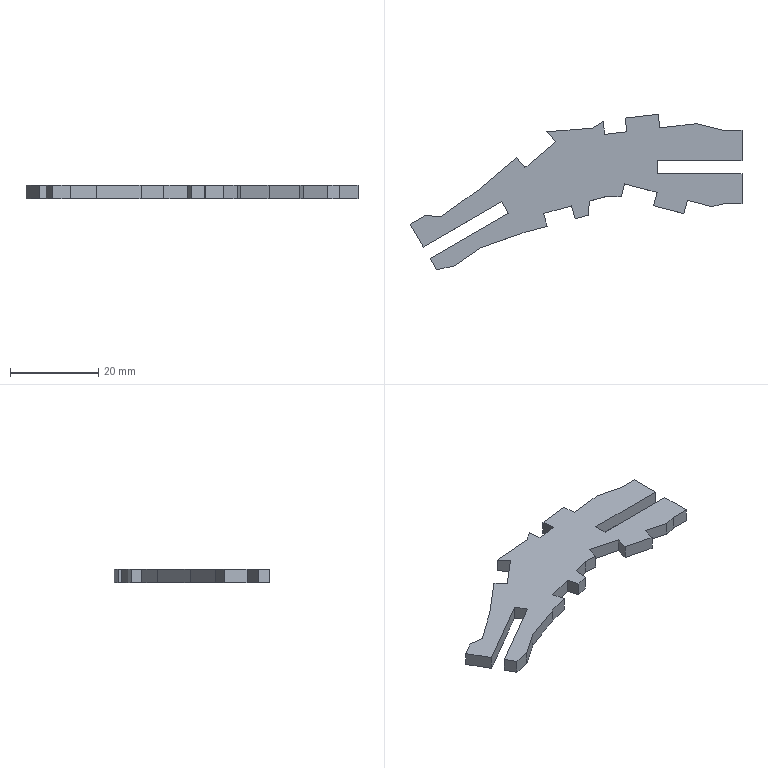Part | SolidWorks | features BaseBody 1 | 1 solid | 48 faces | box 75.297 x 35.268 x 3 mm | volume 3149 mm3 | plane 48
STEP:
#1=CARTESIAN_POINT('',(-41.672,11.926,-1.5));
#2=VERTEX_POINT('',#1);
#3=CARTESIAN_POINT('',(-45.861,11.926,-1.5));
#4=VERTEX_POINT('',#3);
#5=CARTESIAN_POINT('',(0.,11.926,-1.5));
#6=DIRECTION('',(-1.,0.,0.));
#7=VECTOR('',#6,1000.);
#8=LINE('',#5,#7);
#9=EDGE_CURVE('',#2,#4,#8,.T.);
#10=ORIENTED_EDGE('',*,*,#9,.F.);
#11=CARTESIAN_POINT('',(-41.672,5.086,-1.5));
#12=VERTEX_POINT('',#11);
#13=CARTESIAN_POINT('',(-41.672,0.,-1.5));
#14=DIRECTION('',(0.,1.,0.));
#15=VECTOR('',#14,1000.);
#16=LINE('',#13,#15);
#17=EDGE_CURVE('',#12,#2,#16,.T.);
#18=ORIENTED_EDGE('',*,*,#17,.F.);
#19=CARTESIAN_POINT('',(-60.886,5.086,-1.5));
#20=VERTEX_POINT('',#19);
#21=CARTESIAN_POINT('',(0.,5.086,-1.5));
#22=DIRECTION('',(1.,0.,0.));
#23=VECTOR('',#22,1000.);
#24=LINE('',#21,#23);
#25=EDGE_CURVE('',#20,#12,#24,.T.);
#26=ORIENTED_EDGE('',*,*,#25,.F.);
#27=CARTESIAN_POINT('',(-60.886,2.088,-1.5));
#28=VERTEX_POINT('',#27);
#29=CARTESIAN_POINT('',(-60.886,0.,-1.5));
#30=DIRECTION('',(0.,1.,0.));
#31=VECTOR('',#30,1000.);
#32=LINE('',#29,#31);
#33=EDGE_CURVE('',#28,#20,#32,.T.);
#34=ORIENTED_EDGE('',*,*,#33,.F.);
#35=CARTESIAN_POINT('',(-41.672,2.088,-1.5));
#36=VERTEX_POINT('',#35);
#37=CARTESIAN_POINT('',(0.,2.088,-1.5));
#38=DIRECTION('',(-1.,0.,0.));
#39=VECTOR('',#38,1000.);
#40=LINE('',#37,#39);
#41=EDGE_CURVE('',#36,#28,#40,.T.);
#42=ORIENTED_EDGE('',*,*,#41,.F.);
#43=CARTESIAN_POINT('',(-41.672,-4.747,-1.5));
#44=VERTEX_POINT('',#43);
#45=CARTESIAN_POINT('',(-41.672,0.,-1.5));
#46=DIRECTION('',(0.,1.,0.));
#47=VECTOR('',#46,1000.);
#48=LINE('',#45,#47);
#49=EDGE_CURVE('',#44,#36,#48,.T.);
#50=ORIENTED_EDGE('',*,*,#49,.F.);
#51=CARTESIAN_POINT('',(-45.859,-4.748,-1.5));
#52=VERTEX_POINT('',#51);
#53=CARTESIAN_POINT('',(0.0009716,-4.738,-1.5));
#54=DIRECTION('',(1.,0.000205,0.));
#55=VECTOR('',#54,1000.);
#56=LINE('',#53,#55);
#57=EDGE_CURVE('',#52,#44,#56,.T.);
#58=ORIENTED_EDGE('',*,*,#57,.F.);
#59=CARTESIAN_POINT('',(-48.55,-5.367,-1.5));
#60=VERTEX_POINT('',#59);
#61=CARTESIAN_POINT('',(-1.268,5.512,-1.5));
#62=DIRECTION('',(0.9745,0.2242,0.));
#63=VECTOR('',#62,1000.);
#64=LINE('',#61,#63);
#65=EDGE_CURVE('',#60,#52,#64,.T.);
#66=ORIENTED_EDGE('',*,*,#65,.F.);
#67=CARTESIAN_POINT('',(-54.059,-3.94,-1.5));
#68=VERTEX_POINT('',#67);
#69=CARTESIAN_POINT('',(-4.355,-16.813,-1.5));
#70=DIRECTION('',(0.9681,-0.2507,0.));
#71=VECTOR('',#70,1000.);
#72=LINE('',#69,#71);
#73=EDGE_CURVE('',#68,#60,#72,.T.);
#74=ORIENTED_EDGE('',*,*,#73,.F.);
#75=CARTESIAN_POINT('',(-54.841,-6.951,-1.5));
#76=VERTEX_POINT('',#75);
#77=CARTESIAN_POINT('',(-49.682,12.907,-1.5));
#78=DIRECTION('',(0.2514,0.9679,0.));
#79=VECTOR('',#78,1000.);
#80=LINE('',#77,#79);
#81=EDGE_CURVE('',#76,#68,#80,.T.);
#82=ORIENTED_EDGE('',*,*,#81,.F.);
#83=CARTESIAN_POINT('',(-61.711,-5.166,-1.5));
#84=VERTEX_POINT('',#83);
#85=CARTESIAN_POINT('',(-5.159,-19.858,-1.5));
#86=DIRECTION('',(0.9679,-0.2514,0.));
#87=VECTOR('',#86,1000.);
#88=LINE('',#85,#87);
#89=EDGE_CURVE('',#84,#76,#88,.T.);
#90=ORIENTED_EDGE('',*,*,#89,.F.);
#91=CARTESIAN_POINT('',(-60.926,-2.144,-1.5));
#92=VERTEX_POINT('',#91);
#93=CARTESIAN_POINT('',(-56.552,14.692,-1.5));
#94=DIRECTION('',(-0.2514,-0.9679,0.));
#95=VECTOR('',#94,1000.);
#96=LINE('',#93,#95);
#97=EDGE_CURVE('',#92,#84,#96,.T.);
#98=ORIENTED_EDGE('',*,*,#97,.F.);
#99=CARTESIAN_POINT('',(-68.318,-0.224,-1.5));
#100=VERTEX_POINT('',#99);
#101=CARTESIAN_POINT('',(-4.372,-16.833,-1.5));
#102=DIRECTION('',(0.9679,-0.2514,0.));
#103=VECTOR('',#102,1000.);
#104=LINE('',#101,#103);
#105=EDGE_CURVE('',#100,#92,#104,.T.);
#106=ORIENTED_EDGE('',*,*,#105,.F.);
#107=CARTESIAN_POINT('',(-69.072,-3.126,-1.5));
#108=VERTEX_POINT('',#107);
#109=CARTESIAN_POINT('',(-63.946,16.609,-1.5));
#110=DIRECTION('',(0.2514,0.9679,0.));
#111=VECTOR('',#110,1000.);
#112=LINE('',#109,#111);
#113=EDGE_CURVE('',#108,#100,#112,.T.);
#114=ORIENTED_EDGE('',*,*,#113,.F.);
#115=CARTESIAN_POINT('',(-72.167,-3.005,-1.5));
#116=VERTEX_POINT('',#115);
#117=CARTESIAN_POINT('',(-0.2275,-5.818,-1.5));
#118=DIRECTION('',(0.9992,-0.03907,0.));
#119=VECTOR('',#118,1000.);
#120=LINE('',#117,#119);
#121=EDGE_CURVE('',#116,#108,#120,.T.);
#122=ORIENTED_EDGE('',*,*,#121,.F.);
#123=CARTESIAN_POINT('',(-76.273,-4.118,-1.5));
#124=VERTEX_POINT('',#123);
#125=CARTESIAN_POINT('',(-4.178,15.419,-1.5));
#126=DIRECTION('',(0.9652,0.2616,0.));
#127=VECTOR('',#126,1000.);
#128=LINE('',#125,#127);
#129=EDGE_CURVE('',#124,#116,#128,.T.);
#130=ORIENTED_EDGE('',*,*,#129,.F.);
#131=CARTESIAN_POINT('',(-76.559,-7.3,-1.5));
#132=VERTEX_POINT('',#131);
#133=CARTESIAN_POINT('',(-75.296,6.762,-1.5));
#134=DIRECTION('',(0.08944,0.996,0.));
#135=VECTOR('',#134,1000.);
#136=LINE('',#133,#135);
#137=EDGE_CURVE('',#132,#124,#136,.T.);
#138=ORIENTED_EDGE('',*,*,#137,.F.);
#139=CARTESIAN_POINT('',(-79.538,-8.108,-1.5));
#140=VERTEX_POINT('',#139);
#141=CARTESIAN_POINT('',(-3.4,12.538,-1.5));
#142=DIRECTION('',(0.9651,0.2617,0.));
#143=VECTOR('',#142,1000.);
#144=LINE('',#141,#143);
#145=EDGE_CURVE('',#140,#132,#144,.T.);
#146=ORIENTED_EDGE('',*,*,#145,.F.);
#147=CARTESIAN_POINT('',(-80.322,-5.216,-1.5));
#148=VERTEX_POINT('',#147);
#149=CARTESIAN_POINT('',(-76.137,-20.649,-1.5));
#150=DIRECTION('',(0.2617,-0.9651,0.));
#151=VECTOR('',#150,1000.);
#152=LINE('',#149,#151);
#153=EDGE_CURVE('',#148,#140,#152,.T.);
#154=ORIENTED_EDGE('',*,*,#153,.F.);
#155=CARTESIAN_POINT('',(-86.653,-6.933,-1.5));
#156=VERTEX_POINT('',#155);
#157=CARTESIAN_POINT('',(-4.185,15.433,-1.5));
#158=DIRECTION('',(0.9651,0.2617,0.));
#159=VECTOR('',#158,1000.);
#160=LINE('',#157,#159);
#161=EDGE_CURVE('',#156,#148,#160,.T.);
#162=ORIENTED_EDGE('',*,*,#161,.F.);
#163=CARTESIAN_POINT('',(-85.869,-9.824,-1.5));
#164=VERTEX_POINT('',#163);
#165=CARTESIAN_POINT('',(-82.468,-22.366,-1.5));
#166=DIRECTION('',(-0.2617,0.9651,0.));
#167=VECTOR('',#166,1000.);
#168=LINE('',#165,#167);
#169=EDGE_CURVE('',#164,#156,#168,.T.);
#170=ORIENTED_EDGE('',*,*,#169,.F.);
#171=CARTESIAN_POINT('',(-90.886,-11.184,-1.5));
#172=VERTEX_POINT('',#171);
#173=CARTESIAN_POINT('',(-3.398,12.534,-1.5));
#174=DIRECTION('',(0.9652,0.2617,0.));
#175=VECTOR('',#174,1000.);
#176=LINE('',#173,#175);
#177=EDGE_CURVE('',#172,#164,#176,.T.);
#178=ORIENTED_EDGE('',*,*,#177,.F.);
#179=CARTESIAN_POINT('',(-100.892,-14.726,-1.5));
#180=VERTEX_POINT('',#179);
#181=CARTESIAN_POINT('',(-6.601,18.649,-1.5));
#182=DIRECTION('',(0.9427,0.3337,0.));
#183=VECTOR('',#182,1000.);
#184=LINE('',#181,#183);
#185=EDGE_CURVE('',#180,#172,#184,.T.);
#186=ORIENTED_EDGE('',*,*,#185,.F.);
#187=CARTESIAN_POINT('',(-106.899,-18.818,-1.5));
#188=VERTEX_POINT('',#187);
#189=CARTESIAN_POINT('',(-25.128,36.886,-1.5));
#190=DIRECTION('',(0.8265,0.563,0.));
#191=VECTOR('',#190,1000.);
#192=LINE('',#189,#191);
#193=EDGE_CURVE('',#188,#180,#192,.T.);
#194=ORIENTED_EDGE('',*,*,#193,.F.);
#195=CARTESIAN_POINT('',(-110.937,-19.69,-1.5));
#196=VERTEX_POINT('',#195);
#197=CARTESIAN_POINT('',(-0.8769,4.063,-1.5));
#198=DIRECTION('',(0.9775,0.211,0.));
#199=VECTOR('',#198,1000.);
#200=LINE('',#197,#199);
#201=EDGE_CURVE('',#196,#188,#200,.T.);
#202=ORIENTED_EDGE('',*,*,#201,.F.);
#203=CARTESIAN_POINT('',(-112.426,-17.126,-1.5));
#204=VERTEX_POINT('',#203);
#205=CARTESIAN_POINT('',(-91.52,-53.134,-1.5));
#206=DIRECTION('',(0.5021,-0.8648,0.));
#207=VECTOR('',#206,1000.);
#208=LINE('',#205,#207);
#209=EDGE_CURVE('',#204,#196,#208,.T.);
#210=ORIENTED_EDGE('',*,*,#209,.F.);
#211=CARTESIAN_POINT('',(-94.713,-6.827,-1.5));
#212=VERTEX_POINT('',#211);
#213=CARTESIAN_POINT('',(-20.961,36.052,-1.5));
#214=DIRECTION('',(-0.8645,-0.5026,0.));
#215=VECTOR('',#214,1000.);
#216=LINE('',#213,#215);
#217=EDGE_CURVE('',#212,#204,#216,.T.);
#218=ORIENTED_EDGE('',*,*,#217,.F.);
#219=CARTESIAN_POINT('',(-96.219,-4.237,-1.5));
#220=VERTEX_POINT('',#219);
#221=CARTESIAN_POINT('',(-73.752,-42.88,-1.5));
#222=DIRECTION('',(0.5026,-0.8645,0.));
#223=VECTOR('',#222,1000.);
#224=LINE('',#221,#223);
#225=EDGE_CURVE('',#220,#212,#224,.T.);
#226=ORIENTED_EDGE('',*,*,#225,.F.);
#227=CARTESIAN_POINT('',(-113.938,-14.539,-1.5));
#228=VERTEX_POINT('',#227);
#229=CARTESIAN_POINT('',(-22.467,38.642,-1.5));
#230=DIRECTION('',(0.8645,0.5026,0.));
#231=VECTOR('',#230,1000.);
#232=LINE('',#229,#231);
#233=EDGE_CURVE('',#228,#220,#232,.T.);
#234=ORIENTED_EDGE('',*,*,#233,.F.);
#235=CARTESIAN_POINT('',(-116.969,-9.333,-1.5));
#236=VERTEX_POINT('',#235);
#237=CARTESIAN_POINT('',(-91.405,-53.231,-1.5));
#238=DIRECTION('',(0.5032,-0.8641,0.));
#239=VECTOR('',#238,1000.);
#240=LINE('',#237,#239);
#241=EDGE_CURVE('',#236,#228,#240,.T.);
#242=ORIENTED_EDGE('',*,*,#241,.F.);
#243=CARTESIAN_POINT('',(-113.563,-7.354,-1.5));
#244=VERTEX_POINT('',#243);
#245=CARTESIAN_POINT('',(-25.463,43.829,-1.5));
#246=DIRECTION('',(-0.8647,-0.5023,0.));
#247=VECTOR('',#246,1000.);
#248=LINE('',#245,#247);
#249=EDGE_CURVE('',#244,#236,#248,.T.);
#250=ORIENTED_EDGE('',*,*,#249,.F.);
#251=CARTESIAN_POINT('',(-110.024,-7.716,-1.5));
#252=VERTEX_POINT('',#251);
#253=CARTESIAN_POINT('',(-1.92,-18.772,-1.5));
#254=DIRECTION('',(-0.9948,0.1017,0.));
#255=VECTOR('',#254,1000.);
#256=LINE('',#253,#255);
#257=EDGE_CURVE('',#252,#244,#256,.T.);
#258=ORIENTED_EDGE('',*,*,#257,.F.);
#259=CARTESIAN_POINT('',(-101.517,-1.618,-1.5));
#260=VERTEX_POINT('',#259);
#261=CARTESIAN_POINT('',(-33.689,47.,-1.5));
#262=DIRECTION('',(-0.8128,-0.5826,0.));
#263=VECTOR('',#262,1000.);
#264=LINE('',#261,#263);
#265=EDGE_CURVE('',#260,#252,#264,.T.);
#266=ORIENTED_EDGE('',*,*,#265,.F.);
#267=CARTESIAN_POINT('',(-92.851,5.744,-1.5));
#268=VERTEX_POINT('',#267);
#269=CARTESIAN_POINT('',(-41.755,49.151,-1.5));
#270=DIRECTION('',(-0.7621,-0.6474,0.));
#271=VECTOR('',#270,1000.);
#272=LINE('',#269,#271);
#273=EDGE_CURVE('',#268,#260,#272,.T.);
#274=ORIENTED_EDGE('',*,*,#273,.F.);
#275=CARTESIAN_POINT('',(-90.898,3.44,-1.5));
#276=VERTEX_POINT('',#275);
#277=CARTESIAN_POINT('',(-51.19,-43.398,-1.5));
#278=DIRECTION('',(-0.6467,0.7628,0.));
#279=VECTOR('',#278,1000.);
#280=LINE('',#277,#279);
#281=EDGE_CURVE('',#276,#268,#280,.T.);
#282=ORIENTED_EDGE('',*,*,#281,.F.);
#283=CARTESIAN_POINT('',(-83.964,9.318,-1.5));
#284=VERTEX_POINT('',#283);
#285=CARTESIAN_POINT('',(-39.708,46.838,-1.5));
#286=DIRECTION('',(-0.7628,-0.6467,0.));
#287=VECTOR('',#286,1000.);
#288=LINE('',#285,#287);
#289=EDGE_CURVE('',#284,#276,#288,.T.);
#290=ORIENTED_EDGE('',*,*,#289,.F.);
#291=CARTESIAN_POINT('',(-85.9,11.602,-1.5));
#292=VERTEX_POINT('',#291);
#293=CARTESIAN_POINT('',(-44.256,-37.519,-1.5));
#294=DIRECTION('',(0.6467,-0.7628,0.));
#295=VECTOR('',#294,1000.);
#296=LINE('',#293,#295);
#297=EDGE_CURVE('',#292,#284,#296,.T.);
#298=ORIENTED_EDGE('',*,*,#297,.F.);
#299=CARTESIAN_POINT('',(-75.689,12.418,-1.5));
#300=VERTEX_POINT('',#299);
#301=CARTESIAN_POINT('',(-1.467,18.351,-1.5));
#302=DIRECTION('',(-0.9968,-0.07967,0.));
#303=VECTOR('',#302,1000.);
#304=LINE('',#301,#303);
#305=EDGE_CURVE('',#300,#292,#304,.T.);
#306=ORIENTED_EDGE('',*,*,#305,.F.);
#307=CARTESIAN_POINT('',(-73.15,13.963,-1.5));
#308=VERTEX_POINT('',#307);
#309=CARTESIAN_POINT('',(-25.962,42.673,-1.5));
#310=DIRECTION('',(-0.8543,-0.5198,0.));
#311=VECTOR('',#310,1000.);
#312=LINE('',#309,#311);
#313=EDGE_CURVE('',#308,#300,#312,.T.);
#314=ORIENTED_EDGE('',*,*,#313,.F.);
#315=CARTESIAN_POINT('',(-72.806,11.016,-1.5));
#316=VERTEX_POINT('',#315);
#317=CARTESIAN_POINT('',(-70.559,-8.237,-1.5));
#318=DIRECTION('',(-0.116,0.9933,0.));
#319=VECTOR('',#318,1000.);
#320=LINE('',#317,#319);
#321=EDGE_CURVE('',#316,#308,#320,.T.);
#322=ORIENTED_EDGE('',*,*,#321,.F.);
#323=CARTESIAN_POINT('',(-67.808,11.6,-1.5));
#324=VERTEX_POINT('',#323);
#325=CARTESIAN_POINT('',(-2.248,19.253,-1.5));
#326=DIRECTION('',(-0.9933,-0.116,0.));
#327=VECTOR('',#326,1000.);
#328=LINE('',#325,#327);
#329=EDGE_CURVE('',#324,#316,#328,.T.);
#330=ORIENTED_EDGE('',*,*,#329,.F.);
#331=CARTESIAN_POINT('',(-68.17,14.703,-1.5));
#332=VERTEX_POINT('',#331);
#333=CARTESIAN_POINT('',(-65.555,-7.665,-1.5));
#334=DIRECTION('',(0.1161,-0.9932,0.));
#335=VECTOR('',#334,1000.);
#336=LINE('',#333,#335);
#337=EDGE_CURVE('',#332,#324,#336,.T.);
#338=ORIENTED_EDGE('',*,*,#337,.F.);
#339=CARTESIAN_POINT('',(-60.678,15.579,-1.5));
#340=VERTEX_POINT('',#339);
#341=CARTESIAN_POINT('',(-2.615,22.368,-1.5));
#342=DIRECTION('',(-0.9932,-0.1161,0.));
#343=VECTOR('',#342,1000.);
#344=LINE('',#341,#343);
#345=EDGE_CURVE('',#340,#332,#344,.T.);
#346=ORIENTED_EDGE('',*,*,#345,.F.);
#347=CARTESIAN_POINT('',(-60.315,12.476,-1.5));
#348=VERTEX_POINT('',#347);
#349=CARTESIAN_POINT('',(-58.063,-6.789,-1.5));
#350=DIRECTION('',(-0.1161,0.9932,0.));
#351=VECTOR('',#350,1000.);
#352=LINE('',#349,#351);
#353=EDGE_CURVE('',#348,#340,#352,.T.);
#354=ORIENTED_EDGE('',*,*,#353,.F.);
#355=CARTESIAN_POINT('',(-52.074,13.44,-1.5));
#356=VERTEX_POINT('',#355);
#357=CARTESIAN_POINT('',(-2.253,19.265,-1.5));
#358=DIRECTION('',(-0.9932,-0.1161,0.));
#359=VECTOR('',#358,1000.);
#360=LINE('',#357,#359);
#361=EDGE_CURVE('',#356,#348,#360,.T.);
#362=ORIENTED_EDGE('',*,*,#361,.F.);
#363=CARTESIAN_POINT('',(0.1731,0.7104,-1.5));
#364=DIRECTION('',(-0.9716,0.2367,0.));
#365=VECTOR('',#364,1000.);
#366=LINE('',#363,#365);
#367=EDGE_CURVE('',#4,#356,#366,.T.);
#368=ORIENTED_EDGE('',*,*,#367,.F.);
#369=EDGE_LOOP('',(#10,#18,#26,#34,#42,#50,#58,#66,#74,#82,#90,#98,#106,#114,#122,#130,#138,#146,#154,#162,#170,#178,#186,#194,#202,#210,#218,#226,#234,#242,#250,#258,#266,#274,#282,#290,#298,#306,#314,#322,#330,#338,#346,#354,#362,#368));
#370=FACE_OUTER_BOUND('',#369,.T.);
#371=CARTESIAN_POINT('',(0.,0.,-1.5));
#372=DIRECTION('',(0.,0.,1.));
#373=DIRECTION('',(1.,0.,0.));
#374=AXIS2_PLACEMENT_3D('',#371,#372,#373);
#375=PLANE('',#374);
#376=ADVANCED_FACE('',(#370),#375,.F.);
#377=CARTESIAN_POINT('',(-41.672,11.926,1.5));
#378=VERTEX_POINT('',#377);
#379=CARTESIAN_POINT('',(-45.861,11.926,1.5));
#380=VERTEX_POINT('',#379);
#381=CARTESIAN_POINT('',(0.,11.926,1.5));
#382=DIRECTION('',(-1.,0.,0.));
#383=VECTOR('',#382,1000.);
#384=LINE('',#381,#383);
#385=EDGE_CURVE('',#378,#380,#384,.T.);
#386=ORIENTED_EDGE('',*,*,#385,.T.);
#387=CARTESIAN_POINT('',(-52.074,13.44,1.5));
#388=VERTEX_POINT('',#387);
#389=CARTESIAN_POINT('',(0.1731,0.7104,1.5));
#390=DIRECTION('',(-0.9716,0.2367,0.));
#391=VECTOR('',#390,1000.);
#392=LINE('',#389,#391);
#393=EDGE_CURVE('',#380,#388,#392,.T.);
#394=ORIENTED_EDGE('',*,*,#393,.T.);
#395=CARTESIAN_POINT('',(-60.315,12.476,1.5));
#396=VERTEX_POINT('',#395);
#397=CARTESIAN_POINT('',(-2.253,19.265,1.5));
#398=DIRECTION('',(-0.9932,-0.1161,0.));
#399=VECTOR('',#398,1000.);
#400=LINE('',#397,#399);
#401=EDGE_CURVE('',#388,#396,#400,.T.);
#402=ORIENTED_EDGE('',*,*,#401,.T.);
#403=CARTESIAN_POINT('',(-60.678,15.579,1.5));
#404=VERTEX_POINT('',#403);
#405=CARTESIAN_POINT('',(-58.063,-6.789,1.5));
#406=DIRECTION('',(-0.1161,0.9932,0.));
#407=VECTOR('',#406,1000.);
#408=LINE('',#405,#407);
#409=EDGE_CURVE('',#396,#404,#408,.T.);
#410=ORIENTED_EDGE('',*,*,#409,.T.);
#411=CARTESIAN_POINT('',(-68.17,14.703,1.5));
#412=VERTEX_POINT('',#411);
#413=CARTESIAN_POINT('',(-2.615,22.368,1.5));
#414=DIRECTION('',(-0.9932,-0.1161,0.));
#415=VECTOR('',#414,1000.);
#416=LINE('',#413,#415);
#417=EDGE_CURVE('',#404,#412,#416,.T.);
#418=ORIENTED_EDGE('',*,*,#417,.T.);
#419=CARTESIAN_POINT('',(-67.808,11.6,1.5));
#420=VERTEX_POINT('',#419);
#421=CARTESIAN_POINT('',(-65.555,-7.665,1.5));
#422=DIRECTION('',(0.1161,-0.9932,0.));
#423=VECTOR('',#422,1000.);
#424=LINE('',#421,#423);
#425=EDGE_CURVE('',#412,#420,#424,.T.);
#426=ORIENTED_EDGE('',*,*,#425,.T.);
#427=CARTESIAN_POINT('',(-72.806,11.016,1.5));
#428=VERTEX_POINT('',#427);
#429=CARTESIAN_POINT('',(-2.248,19.253,1.5));
#430=DIRECTION('',(-0.9933,-0.116,0.));
#431=VECTOR('',#430,1000.);
#432=LINE('',#429,#431);
#433=EDGE_CURVE('',#420,#428,#432,.T.);
#434=ORIENTED_EDGE('',*,*,#433,.T.);
#435=CARTESIAN_POINT('',(-73.15,13.963,1.5));
#436=VERTEX_POINT('',#435);
#437=CARTESIAN_POINT('',(-70.559,-8.237,1.5));
#438=DIRECTION('',(-0.116,0.9933,0.));
#439=VECTOR('',#438,1000.);
#440=LINE('',#437,#439);
#441=EDGE_CURVE('',#428,#436,#440,.T.);
#442=ORIENTED_EDGE('',*,*,#441,.T.);
#443=CARTESIAN_POINT('',(-75.689,12.418,1.5));
#444=VERTEX_POINT('',#443);
#445=CARTESIAN_POINT('',(-25.962,42.673,1.5));
#446=DIRECTION('',(-0.8543,-0.5198,0.));
#447=VECTOR('',#446,1000.);
#448=LINE('',#445,#447);
#449=EDGE_CURVE('',#436,#444,#448,.T.);
#450=ORIENTED_EDGE('',*,*,#449,.T.);
#451=CARTESIAN_POINT('',(-85.9,11.602,1.5));
#452=VERTEX_POINT('',#451);
#453=CARTESIAN_POINT('',(-1.467,18.351,1.5));
#454=DIRECTION('',(-0.9968,-0.07967,0.));
#455=VECTOR('',#454,1000.);
#456=LINE('',#453,#455);
#457=EDGE_CURVE('',#444,#452,#456,.T.);
#458=ORIENTED_EDGE('',*,*,#457,.T.);
#459=CARTESIAN_POINT('',(-83.964,9.318,1.5));
#460=VERTEX_POINT('',#459);
#461=CARTESIAN_POINT('',(-44.256,-37.519,1.5));
#462=DIRECTION('',(0.6467,-0.7628,0.));
#463=VECTOR('',#462,1000.);
#464=LINE('',#461,#463);
#465=EDGE_CURVE('',#452,#460,#464,.T.);
#466=ORIENTED_EDGE('',*,*,#465,.T.);
#467=CARTESIAN_POINT('',(-90.898,3.44,1.5));
#468=VERTEX_POINT('',#467);
#469=CARTESIAN_POINT('',(-39.708,46.838,1.5));
#470=DIRECTION('',(-0.7628,-0.6467,0.));
#471=VECTOR('',#470,1000.);
#472=LINE('',#469,#471);
#473=EDGE_CURVE('',#460,#468,#472,.T.);
#474=ORIENTED_EDGE('',*,*,#473,.T.);
#475=CARTESIAN_POINT('',(-92.851,5.744,1.5));
#476=VERTEX_POINT('',#475);
#477=CARTESIAN_POINT('',(-51.19,-43.398,1.5));
#478=DIRECTION('',(-0.6467,0.7628,0.));
#479=VECTOR('',#478,1000.);
#480=LINE('',#477,#479);
#481=EDGE_CURVE('',#468,#476,#480,.T.);
#482=ORIENTED_EDGE('',*,*,#481,.T.);
#483=CARTESIAN_POINT('',(-101.517,-1.618,1.5));
#484=VERTEX_POINT('',#483);
#485=CARTESIAN_POINT('',(-41.755,49.151,1.5));
#486=DIRECTION('',(-0.7621,-0.6474,0.));
#487=VECTOR('',#486,1000.);
#488=LINE('',#485,#487);
#489=EDGE_CURVE('',#476,#484,#488,.T.);
#490=ORIENTED_EDGE('',*,*,#489,.T.);
#491=CARTESIAN_POINT('',(-110.024,-7.716,1.5));
#492=VERTEX_POINT('',#491);
#493=CARTESIAN_POINT('',(-33.689,47.,1.5));
#494=DIRECTION('',(-0.8128,-0.5826,0.));
#495=VECTOR('',#494,1000.);
#496=LINE('',#493,#495);
#497=EDGE_CURVE('',#484,#492,#496,.T.);
#498=ORIENTED_EDGE('',*,*,#497,.T.);
#499=CARTESIAN_POINT('',(-113.563,-7.354,1.5));
#500=VERTEX_POINT('',#499);
#501=CARTESIAN_POINT('',(-1.92,-18.772,1.5));
#502=DIRECTION('',(-0.9948,0.1017,0.));
#503=VECTOR('',#502,1000.);
#504=LINE('',#501,#503);
#505=EDGE_CURVE('',#492,#500,#504,.T.);
#506=ORIENTED_EDGE('',*,*,#505,.T.);
#507=CARTESIAN_POINT('',(-116.969,-9.333,1.5));
#508=VERTEX_POINT('',#507);
#509=CARTESIAN_POINT('',(-25.463,43.829,1.5));
#510=DIRECTION('',(-0.8647,-0.5023,0.));
#511=VECTOR('',#510,1000.);
#512=LINE('',#509,#511);
#513=EDGE_CURVE('',#500,#508,#512,.T.);
#514=ORIENTED_EDGE('',*,*,#513,.T.);
#515=CARTESIAN_POINT('',(-113.938,-14.539,1.5));
#516=VERTEX_POINT('',#515);
#517=CARTESIAN_POINT('',(-91.405,-53.231,1.5));
#518=DIRECTION('',(0.5032,-0.8641,0.));
#519=VECTOR('',#518,1000.);
#520=LINE('',#517,#519);
#521=EDGE_CURVE('',#508,#516,#520,.T.);
#522=ORIENTED_EDGE('',*,*,#521,.T.);
#523=CARTESIAN_POINT('',(-96.219,-4.237,1.5));
#524=VERTEX_POINT('',#523);
#525=CARTESIAN_POINT('',(-22.467,38.642,1.5));
#526=DIRECTION('',(0.8645,0.5026,0.));
#527=VECTOR('',#526,1000.);
#528=LINE('',#525,#527);
#529=EDGE_CURVE('',#516,#524,#528,.T.);
#530=ORIENTED_EDGE('',*,*,#529,.T.);
#531=CARTESIAN_POINT('',(-94.713,-6.827,1.5));
#532=VERTEX_POINT('',#531);
#533=CARTESIAN_POINT('',(-73.752,-42.88,1.5));
#534=DIRECTION('',(0.5026,-0.8645,0.));
#535=VECTOR('',#534,1000.);
#536=LINE('',#533,#535);
#537=EDGE_CURVE('',#524,#532,#536,.T.);
#538=ORIENTED_EDGE('',*,*,#537,.T.);
#539=CARTESIAN_POINT('',(-112.426,-17.126,1.5));
#540=VERTEX_POINT('',#539);
#541=CARTESIAN_POINT('',(-20.961,36.052,1.5));
#542=DIRECTION('',(-0.8645,-0.5026,0.));
#543=VECTOR('',#542,1000.);
#544=LINE('',#541,#543);
#545=EDGE_CURVE('',#532,#540,#544,.T.);
#546=ORIENTED_EDGE('',*,*,#545,.T.);
#547=CARTESIAN_POINT('',(-110.937,-19.69,1.5));
#548=VERTEX_POINT('',#547);
#549=CARTESIAN_POINT('',(-91.52,-53.134,1.5));
#550=DIRECTION('',(0.5021,-0.8648,0.));
#551=VECTOR('',#550,1000.);
#552=LINE('',#549,#551);
#553=EDGE_CURVE('',#540,#548,#552,.T.);
#554=ORIENTED_EDGE('',*,*,#553,.T.);
#555=CARTESIAN_POINT('',(-106.899,-18.818,1.5));
#556=VERTEX_POINT('',#555);
#557=CARTESIAN_POINT('',(-0.8769,4.063,1.5));
#558=DIRECTION('',(0.9775,0.211,0.));
#559=VECTOR('',#558,1000.);
#560=LINE('',#557,#559);
#561=EDGE_CURVE('',#548,#556,#560,.T.);
#562=ORIENTED_EDGE('',*,*,#561,.T.);
#563=CARTESIAN_POINT('',(-100.892,-14.726,1.5));
#564=VERTEX_POINT('',#563);
#565=CARTESIAN_POINT('',(-25.128,36.886,1.5));
#566=DIRECTION('',(0.8265,0.563,0.));
#567=VECTOR('',#566,1000.);
#568=LINE('',#565,#567);
#569=EDGE_CURVE('',#556,#564,#568,.T.);
#570=ORIENTED_EDGE('',*,*,#569,.T.);
#571=CARTESIAN_POINT('',(-90.886,-11.184,1.5));
#572=VERTEX_POINT('',#571);
#573=CARTESIAN_POINT('',(-6.601,18.649,1.5));
#574=DIRECTION('',(0.9427,0.3337,0.));
#575=VECTOR('',#574,1000.);
#576=LINE('',#573,#575);
#577=EDGE_CURVE('',#564,#572,#576,.T.);
#578=ORIENTED_EDGE('',*,*,#577,.T.);
#579=CARTESIAN_POINT('',(-85.869,-9.824,1.5));
#580=VERTEX_POINT('',#579);
#581=CARTESIAN_POINT('',(-3.398,12.534,1.5));
#582=DIRECTION('',(0.9652,0.2617,0.));
#583=VECTOR('',#582,1000.);
#584=LINE('',#581,#583);
#585=EDGE_CURVE('',#572,#580,#584,.T.);
#586=ORIENTED_EDGE('',*,*,#585,.T.);
#587=CARTESIAN_POINT('',(-86.653,-6.933,1.5));
#588=VERTEX_POINT('',#587);
#589=CARTESIAN_POINT('',(-82.468,-22.366,1.5));
#590=DIRECTION('',(-0.2617,0.9651,0.));
#591=VECTOR('',#590,1000.);
#592=LINE('',#589,#591);
#593=EDGE_CURVE('',#580,#588,#592,.T.);
#594=ORIENTED_EDGE('',*,*,#593,.T.);
#595=CARTESIAN_POINT('',(-80.322,-5.216,1.5));
#596=VERTEX_POINT('',#595);
#597=CARTESIAN_POINT('',(-4.185,15.433,1.5));
#598=DIRECTION('',(0.9651,0.2617,0.));
#599=VECTOR('',#598,1000.);
#600=LINE('',#597,#599);
#601=EDGE_CURVE('',#588,#596,#600,.T.);
#602=ORIENTED_EDGE('',*,*,#601,.T.);
#603=CARTESIAN_POINT('',(-79.538,-8.108,1.5));
#604=VERTEX_POINT('',#603);
#605=CARTESIAN_POINT('',(-76.137,-20.649,1.5));
#606=DIRECTION('',(0.2617,-0.9651,0.));
#607=VECTOR('',#606,1000.);
#608=LINE('',#605,#607);
#609=EDGE_CURVE('',#596,#604,#608,.T.);
#610=ORIENTED_EDGE('',*,*,#609,.T.);
#611=CARTESIAN_POINT('',(-76.559,-7.3,1.5));
#612=VERTEX_POINT('',#611);
#613=CARTESIAN_POINT('',(-3.4,12.538,1.5));
#614=DIRECTION('',(0.9651,0.2617,0.));
#615=VECTOR('',#614,1000.);
#616=LINE('',#613,#615);
#617=EDGE_CURVE('',#604,#612,#616,.T.);
#618=ORIENTED_EDGE('',*,*,#617,.T.);
#619=CARTESIAN_POINT('',(-76.273,-4.118,1.5));
#620=VERTEX_POINT('',#619);
#621=CARTESIAN_POINT('',(-75.296,6.762,1.5));
#622=DIRECTION('',(0.08944,0.996,0.));
#623=VECTOR('',#622,1000.);
#624=LINE('',#621,#623);
#625=EDGE_CURVE('',#612,#620,#624,.T.);
#626=ORIENTED_EDGE('',*,*,#625,.T.);
#627=CARTESIAN_POINT('',(-72.167,-3.005,1.5));
#628=VERTEX_POINT('',#627);
#629=CARTESIAN_POINT('',(-4.178,15.419,1.5));
#630=DIRECTION('',(0.9652,0.2616,0.));
#631=VECTOR('',#630,1000.);
#632=LINE('',#629,#631);
#633=EDGE_CURVE('',#620,#628,#632,.T.);
#634=ORIENTED_EDGE('',*,*,#633,.T.);
#635=CARTESIAN_POINT('',(-69.072,-3.126,1.5));
#636=VERTEX_POINT('',#635);
#637=CARTESIAN_POINT('',(-0.2275,-5.818,1.5));
#638=DIRECTION('',(0.9992,-0.03907,0.));
#639=VECTOR('',#638,1000.);
#640=LINE('',#637,#639);
#641=EDGE_CURVE('',#628,#636,#640,.T.);
#642=ORIENTED_EDGE('',*,*,#641,.T.);
#643=CARTESIAN_POINT('',(-68.318,-0.224,1.5));
#644=VERTEX_POINT('',#643);
#645=CARTESIAN_POINT('',(-63.946,16.609,1.5));
#646=DIRECTION('',(0.2514,0.9679,0.));
#647=VECTOR('',#646,1000.);
#648=LINE('',#645,#647);
#649=EDGE_CURVE('',#636,#644,#648,.T.);
#650=ORIENTED_EDGE('',*,*,#649,.T.);
#651=CARTESIAN_POINT('',(-60.926,-2.144,1.5));
#652=VERTEX_POINT('',#651);
#653=CARTESIAN_POINT('',(-4.372,-16.833,1.5));
#654=DIRECTION('',(0.9679,-0.2514,0.));
#655=VECTOR('',#654,1000.);
#656=LINE('',#653,#655);
#657=EDGE_CURVE('',#644,#652,#656,.T.);
#658=ORIENTED_EDGE('',*,*,#657,.T.);
#659=CARTESIAN_POINT('',(-61.711,-5.166,1.5));
#660=VERTEX_POINT('',#659);
#661=CARTESIAN_POINT('',(-56.552,14.692,1.5));
#662=DIRECTION('',(-0.2514,-0.9679,0.));
#663=VECTOR('',#662,1000.);
#664=LINE('',#661,#663);
#665=EDGE_CURVE('',#652,#660,#664,.T.);
#666=ORIENTED_EDGE('',*,*,#665,.T.);
#667=CARTESIAN_POINT('',(-54.841,-6.951,1.5));
#668=VERTEX_POINT('',#667);
#669=CARTESIAN_POINT('',(-5.159,-19.858,1.5));
#670=DIRECTION('',(0.9679,-0.2514,0.));
#671=VECTOR('',#670,1000.);
#672=LINE('',#669,#671);
#673=EDGE_CURVE('',#660,#668,#672,.T.);
#674=ORIENTED_EDGE('',*,*,#673,.T.);
#675=CARTESIAN_POINT('',(-54.059,-3.94,1.5));
#676=VERTEX_POINT('',#675);
#677=CARTESIAN_POINT('',(-49.682,12.907,1.5));
#678=DIRECTION('',(0.2514,0.9679,0.));
#679=VECTOR('',#678,1000.);
#680=LINE('',#677,#679);
#681=EDGE_CURVE('',#668,#676,#680,.T.);
#682=ORIENTED_EDGE('',*,*,#681,.T.);
#683=CARTESIAN_POINT('',(-48.55,-5.367,1.5));
#684=VERTEX_POINT('',#683);
#685=CARTESIAN_POINT('',(-4.355,-16.813,1.5));
#686=DIRECTION('',(0.9681,-0.2507,0.));
#687=VECTOR('',#686,1000.);
#688=LINE('',#685,#687);
#689=EDGE_CURVE('',#676,#684,#688,.T.);
#690=ORIENTED_EDGE('',*,*,#689,.T.);
#691=CARTESIAN_POINT('',(-45.859,-4.748,1.5));
#692=VERTEX_POINT('',#691);
#693=CARTESIAN_POINT('',(-1.268,5.512,1.5));
#694=DIRECTION('',(0.9745,0.2242,0.));
#695=VECTOR('',#694,1000.);
#696=LINE('',#693,#695);
#697=EDGE_CURVE('',#684,#692,#696,.T.);
#698=ORIENTED_EDGE('',*,*,#697,.T.);
#699=CARTESIAN_POINT('',(-41.672,-4.747,1.5));
#700=VERTEX_POINT('',#699);
#701=CARTESIAN_POINT('',(0.0009716,-4.738,1.5));
#702=DIRECTION('',(1.,0.000205,0.));
#703=VECTOR('',#702,1000.);
#704=LINE('',#701,#703);
#705=EDGE_CURVE('',#692,#700,#704,.T.);
#706=ORIENTED_EDGE('',*,*,#705,.T.);
#707=CARTESIAN_POINT('',(-41.672,2.088,1.5));
#708=VERTEX_POINT('',#707);
#709=CARTESIAN_POINT('',(-41.672,0.,1.5));
#710=DIRECTION('',(0.,1.,0.));
#711=VECTOR('',#710,1000.);
#712=LINE('',#709,#711);
#713=EDGE_CURVE('',#700,#708,#712,.T.);
#714=ORIENTED_EDGE('',*,*,#713,.T.);
#715=CARTESIAN_POINT('',(-60.886,2.088,1.5));
#716=VERTEX_POINT('',#715);
#717=CARTESIAN_POINT('',(0.,2.088,1.5));
#718=DIRECTION('',(-1.,0.,0.));
#719=VECTOR('',#718,1000.);
#720=LINE('',#717,#719);
#721=EDGE_CURVE('',#708,#716,#720,.T.);
#722=ORIENTED_EDGE('',*,*,#721,.T.);
#723=CARTESIAN_POINT('',(-60.886,5.086,1.5));
#724=VERTEX_POINT('',#723);
#725=CARTESIAN_POINT('',(-60.886,0.,1.5));
#726=DIRECTION('',(0.,1.,0.));
#727=VECTOR('',#726,1000.);
#728=LINE('',#725,#727);
#729=EDGE_CURVE('',#716,#724,#728,.T.);
#730=ORIENTED_EDGE('',*,*,#729,.T.);
#731=CARTESIAN_POINT('',(-41.672,5.086,1.5));
#732=VERTEX_POINT('',#731);
#733=CARTESIAN_POINT('',(0.,5.086,1.5));
#734=DIRECTION('',(1.,0.,0.));
#735=VECTOR('',#734,1000.);
#736=LINE('',#733,#735);
#737=EDGE_CURVE('',#724,#732,#736,.T.);
#738=ORIENTED_EDGE('',*,*,#737,.T.);
#739=CARTESIAN_POINT('',(-41.672,0.,1.5));
#740=DIRECTION('',(0.,1.,0.));
#741=VECTOR('',#740,1000.);
#742=LINE('',#739,#741);
#743=EDGE_CURVE('',#732,#378,#742,.T.);
#744=ORIENTED_EDGE('',*,*,#743,.T.);
#745=EDGE_LOOP('',(#386,#394,#402,#410,#418,#426,#434,#442,#450,#458,#466,#474,#482,#490,#498,#506,#514,#522,#530,#538,#546,#554,#562,#570,#578,#586,#594,#602,#610,#618,#626,#634,#642,#650,#658,#666,#674,#682,#690,#698,#706,#714,#722,#730,#738,#744));
#746=FACE_OUTER_BOUND('',#745,.T.);
#747=CARTESIAN_POINT('',(0.,0.,1.5));
#748=DIRECTION('',(0.,0.,1.));
#749=DIRECTION('',(1.,0.,0.));
#750=AXIS2_PLACEMENT_3D('',#747,#748,#749);
#751=PLANE('',#750);
#752=ADVANCED_FACE('',(#746),#751,.T.);
#753=ORIENTED_EDGE('',*,*,#17,.T.);
#754=CARTESIAN_POINT('',(-41.672,11.926,1.5));
#755=DIRECTION('',(0.,0.,-1.));
#756=VECTOR('',#755,1000.);
#757=LINE('',#754,#756);
#758=EDGE_CURVE('',#378,#2,#757,.T.);
#759=ORIENTED_EDGE('',*,*,#758,.F.);
#760=ORIENTED_EDGE('',*,*,#743,.F.);
#761=CARTESIAN_POINT('',(-41.672,5.086,1.5));
#762=DIRECTION('',(0.,0.,-1.));
#763=VECTOR('',#762,1000.);
#764=LINE('',#761,#763);
#765=EDGE_CURVE('',#732,#12,#764,.T.);
#766=ORIENTED_EDGE('',*,*,#765,.T.);
#767=EDGE_LOOP('',(#753,#759,#760,#766));
#768=FACE_OUTER_BOUND('',#767,.T.);
#769=CARTESIAN_POINT('',(-41.672,0.,1.5));
#770=DIRECTION('',(-1.,0.,0.));
#771=DIRECTION('',(0.,1.,0.));
#772=AXIS2_PLACEMENT_3D('',#769,#770,#771);
#773=PLANE('',#772);
#774=ADVANCED_FACE('',(#768),#773,.F.);
#775=ORIENTED_EDGE('',*,*,#25,.T.);
#776=ORIENTED_EDGE('',*,*,#765,.F.);
#777=ORIENTED_EDGE('',*,*,#737,.F.);
#778=CARTESIAN_POINT('',(-60.886,5.086,1.5));
#779=DIRECTION('',(0.,0.,-1.));
#780=VECTOR('',#779,1000.);
#781=LINE('',#778,#780);
#782=EDGE_CURVE('',#724,#20,#781,.T.);
#783=ORIENTED_EDGE('',*,*,#782,.T.);
#784=EDGE_LOOP('',(#775,#776,#777,#783));
#785=FACE_OUTER_BOUND('',#784,.T.);
#786=CARTESIAN_POINT('',(0.,5.086,1.5));
#787=DIRECTION('',(0.,1.,0.));
#788=DIRECTION('',(1.,0.,0.));
#789=AXIS2_PLACEMENT_3D('',#786,#787,#788);
#790=PLANE('',#789);
#791=ADVANCED_FACE('',(#785),#790,.F.);
#792=ORIENTED_EDGE('',*,*,#33,.T.);
#793=ORIENTED_EDGE('',*,*,#782,.F.);
#794=ORIENTED_EDGE('',*,*,#729,.F.);
#795=CARTESIAN_POINT('',(-60.886,2.088,1.5));
#796=DIRECTION('',(0.,0.,-1.));
#797=VECTOR('',#796,1000.);
#798=LINE('',#795,#797);
#799=EDGE_CURVE('',#716,#28,#798,.T.);
#800=ORIENTED_EDGE('',*,*,#799,.T.);
#801=EDGE_LOOP('',(#792,#793,#794,#800));
#802=FACE_OUTER_BOUND('',#801,.T.);
#803=CARTESIAN_POINT('',(-60.886,0.,1.5));
#804=DIRECTION('',(-1.,0.,0.));
#805=DIRECTION('',(0.,0.,1.));
#806=AXIS2_PLACEMENT_3D('',#803,#804,#805);
#807=PLANE('',#806);
#808=ADVANCED_FACE('',(#802),#807,.F.);
#809=ORIENTED_EDGE('',*,*,#41,.T.);
#810=ORIENTED_EDGE('',*,*,#799,.F.);
#811=ORIENTED_EDGE('',*,*,#721,.F.);
#812=CARTESIAN_POINT('',(-41.672,2.088,1.5));
#813=DIRECTION('',(0.,0.,-1.));
#814=VECTOR('',#813,1000.);
#815=LINE('',#812,#814);
#816=EDGE_CURVE('',#708,#36,#815,.T.);
#817=ORIENTED_EDGE('',*,*,#816,.T.);
#818=EDGE_LOOP('',(#809,#810,#811,#817));
#819=FACE_OUTER_BOUND('',#818,.T.);
#820=CARTESIAN_POINT('',(0.,2.088,1.5));
#821=DIRECTION('',(0.,-1.,0.));
#822=DIRECTION('',(0.,0.,-1.));
#823=AXIS2_PLACEMENT_3D('',#820,#821,#822);
#824=PLANE('',#823);
#825=ADVANCED_FACE('',(#819),#824,.F.);
#826=ORIENTED_EDGE('',*,*,#49,.T.);
#827=ORIENTED_EDGE('',*,*,#816,.F.);
#828=ORIENTED_EDGE('',*,*,#713,.F.);
#829=CARTESIAN_POINT('',(-41.672,-4.747,1.5));
#830=DIRECTION('',(0.,0.,-1.));
#831=VECTOR('',#830,1000.);
#832=LINE('',#829,#831);
#833=EDGE_CURVE('',#700,#44,#832,.T.);
#834=ORIENTED_EDGE('',*,*,#833,.T.);
#835=EDGE_LOOP('',(#826,#827,#828,#834));
#836=FACE_OUTER_BOUND('',#835,.T.);
#837=CARTESIAN_POINT('',(-41.672,0.,1.5));
#838=DIRECTION('',(-1.,0.,0.));
#839=DIRECTION('',(0.,0.,1.));
#840=AXIS2_PLACEMENT_3D('',#837,#838,#839);
#841=PLANE('',#840);
#842=ADVANCED_FACE('',(#836),#841,.F.);
#843=ORIENTED_EDGE('',*,*,#57,.T.);
#844=ORIENTED_EDGE('',*,*,#833,.F.);
#845=ORIENTED_EDGE('',*,*,#705,.F.);
#846=CARTESIAN_POINT('',(-45.859,-4.748,1.5));
#847=DIRECTION('',(0.,0.,-1.));
#848=VECTOR('',#847,1000.);
#849=LINE('',#846,#848);
#850=EDGE_CURVE('',#692,#52,#849,.T.);
#851=ORIENTED_EDGE('',*,*,#850,.T.);
#852=EDGE_LOOP('',(#843,#844,#845,#851));
#853=FACE_OUTER_BOUND('',#852,.T.);
#854=CARTESIAN_POINT('',(0.0009716,-4.738,1.5));
#855=DIRECTION('',(-0.000205,1.,0.));
#856=DIRECTION('',(0.,0.,1.));
#857=AXIS2_PLACEMENT_3D('',#854,#855,#856);
#858=PLANE('',#857);
#859=ADVANCED_FACE('',(#853),#858,.F.);
#860=ORIENTED_EDGE('',*,*,#65,.T.);
#861=ORIENTED_EDGE('',*,*,#850,.F.);
#862=ORIENTED_EDGE('',*,*,#697,.F.);
#863=CARTESIAN_POINT('',(-48.55,-5.367,1.5));
#864=DIRECTION('',(0.,0.,-1.));
#865=VECTOR('',#864,1000.);
#866=LINE('',#863,#865);
#867=EDGE_CURVE('',#684,#60,#866,.T.);
#868=ORIENTED_EDGE('',*,*,#867,.T.);
#869=EDGE_LOOP('',(#860,#861,#862,#868));
#870=FACE_OUTER_BOUND('',#869,.T.);
#871=CARTESIAN_POINT('',(-1.268,5.512,1.5));
#872=DIRECTION('',(-0.2242,0.9745,0.));
#873=DIRECTION('',(0.,0.,1.));
#874=AXIS2_PLACEMENT_3D('',#871,#872,#873);
#875=PLANE('',#874);
#876=ADVANCED_FACE('',(#870),#875,.F.);
#877=ORIENTED_EDGE('',*,*,#73,.T.);
#878=ORIENTED_EDGE('',*,*,#867,.F.);
#879=ORIENTED_EDGE('',*,*,#689,.F.);
#880=CARTESIAN_POINT('',(-54.059,-3.94,1.5));
#881=DIRECTION('',(0.,0.,-1.));
#882=VECTOR('',#881,1000.);
#883=LINE('',#880,#882);
#884=EDGE_CURVE('',#676,#68,#883,.T.);
#885=ORIENTED_EDGE('',*,*,#884,.T.);
#886=EDGE_LOOP('',(#877,#878,#879,#885));
#887=FACE_OUTER_BOUND('',#886,.T.);
#888=CARTESIAN_POINT('',(-4.355,-16.813,1.5));
#889=DIRECTION('',(0.2507,0.9681,0.));
#890=DIRECTION('',(0.,0.,-1.));
#891=AXIS2_PLACEMENT_3D('',#888,#889,#890);
#892=PLANE('',#891);
#893=ADVANCED_FACE('',(#887),#892,.F.);
#894=ORIENTED_EDGE('',*,*,#81,.T.);
#895=ORIENTED_EDGE('',*,*,#884,.F.);
#896=ORIENTED_EDGE('',*,*,#681,.F.);
#897=CARTESIAN_POINT('',(-54.841,-6.951,1.5));
#898=DIRECTION('',(0.,0.,-1.));
#899=VECTOR('',#898,1000.);
#900=LINE('',#897,#899);
#901=EDGE_CURVE('',#668,#76,#900,.T.);
#902=ORIENTED_EDGE('',*,*,#901,.T.);
#903=EDGE_LOOP('',(#894,#895,#896,#902));
#904=FACE_OUTER_BOUND('',#903,.T.);
#905=CARTESIAN_POINT('',(-49.682,12.907,1.5));
#906=DIRECTION('',(-0.9679,0.2514,0.));
#907=DIRECTION('',(0.,0.,1.));
#908=AXIS2_PLACEMENT_3D('',#905,#906,#907);
#909=PLANE('',#908);
#910=ADVANCED_FACE('',(#904),#909,.F.);
#911=ORIENTED_EDGE('',*,*,#89,.T.);
#912=ORIENTED_EDGE('',*,*,#901,.F.);
#913=ORIENTED_EDGE('',*,*,#673,.F.);
#914=CARTESIAN_POINT('',(-61.711,-5.166,1.5));
#915=DIRECTION('',(0.,0.,-1.));
#916=VECTOR('',#915,1000.);
#917=LINE('',#914,#916);
#918=EDGE_CURVE('',#660,#84,#917,.T.);
#919=ORIENTED_EDGE('',*,*,#918,.T.);
#920=EDGE_LOOP('',(#911,#912,#913,#919));
#921=FACE_OUTER_BOUND('',#920,.T.);
#922=CARTESIAN_POINT('',(-5.159,-19.858,1.5));
#923=DIRECTION('',(0.2514,0.9679,0.));
#924=DIRECTION('',(0.,0.,-1.));
#925=AXIS2_PLACEMENT_3D('',#922,#923,#924);
#926=PLANE('',#925);
#927=ADVANCED_FACE('',(#921),#926,.F.);
#928=ORIENTED_EDGE('',*,*,#97,.T.);
#929=ORIENTED_EDGE('',*,*,#918,.F.);
#930=ORIENTED_EDGE('',*,*,#665,.F.);
#931=CARTESIAN_POINT('',(-60.926,-2.144,1.5));
#932=DIRECTION('',(0.,0.,-1.));
#933=VECTOR('',#932,1000.);
#934=LINE('',#931,#933);
#935=EDGE_CURVE('',#652,#92,#934,.T.);
#936=ORIENTED_EDGE('',*,*,#935,.T.);
#937=EDGE_LOOP('',(#928,#929,#930,#936));
#938=FACE_OUTER_BOUND('',#937,.T.);
#939=CARTESIAN_POINT('',(-56.552,14.692,1.5));
#940=DIRECTION('',(0.9679,-0.2514,0.));
#941=DIRECTION('',(0.,0.,-1.));
#942=AXIS2_PLACEMENT_3D('',#939,#940,#941);
#943=PLANE('',#942);
#944=ADVANCED_FACE('',(#938),#943,.F.);
#945=ORIENTED_EDGE('',*,*,#105,.T.);
#946=ORIENTED_EDGE('',*,*,#935,.F.);
#947=ORIENTED_EDGE('',*,*,#657,.F.);
#948=CARTESIAN_POINT('',(-68.318,-0.224,1.5));
#949=DIRECTION('',(0.,0.,-1.));
#950=VECTOR('',#949,1000.);
#951=LINE('',#948,#950);
#952=EDGE_CURVE('',#644,#100,#951,.T.);
#953=ORIENTED_EDGE('',*,*,#952,.T.);
#954=EDGE_LOOP('',(#945,#946,#947,#953));
#955=FACE_OUTER_BOUND('',#954,.T.);
#956=CARTESIAN_POINT('',(-4.372,-16.833,1.5));
#957=DIRECTION('',(0.2514,0.9679,0.));
#958=DIRECTION('',(0.,0.,-1.));
#959=AXIS2_PLACEMENT_3D('',#956,#957,#958);
#960=PLANE('',#959);
#961=ADVANCED_FACE('',(#955),#960,.F.);
#962=ORIENTED_EDGE('',*,*,#113,.T.);
#963=ORIENTED_EDGE('',*,*,#952,.F.);
#964=ORIENTED_EDGE('',*,*,#649,.F.);
#965=CARTESIAN_POINT('',(-69.072,-3.126,1.5));
#966=DIRECTION('',(0.,0.,-1.));
#967=VECTOR('',#966,1000.);
#968=LINE('',#965,#967);
#969=EDGE_CURVE('',#636,#108,#968,.T.);
#970=ORIENTED_EDGE('',*,*,#969,.T.);
#971=EDGE_LOOP('',(#962,#963,#964,#970));
#972=FACE_OUTER_BOUND('',#971,.T.);
#973=CARTESIAN_POINT('',(-63.946,16.609,1.5));
#974=DIRECTION('',(-0.9679,0.2514,0.));
#975=DIRECTION('',(0.,0.,1.));
#976=AXIS2_PLACEMENT_3D('',#973,#974,#975);
#977=PLANE('',#976);
#978=ADVANCED_FACE('',(#972),#977,.F.);
#979=ORIENTED_EDGE('',*,*,#121,.T.);
#980=ORIENTED_EDGE('',*,*,#969,.F.);
#981=ORIENTED_EDGE('',*,*,#641,.F.);
#982=CARTESIAN_POINT('',(-72.167,-3.005,1.5));
#983=DIRECTION('',(0.,0.,-1.));
#984=VECTOR('',#983,1000.);
#985=LINE('',#982,#984);
#986=EDGE_CURVE('',#628,#116,#985,.T.);
#987=ORIENTED_EDGE('',*,*,#986,.T.);
#988=EDGE_LOOP('',(#979,#980,#981,#987));
#989=FACE_OUTER_BOUND('',#988,.T.);
#990=CARTESIAN_POINT('',(-0.2275,-5.818,1.5));
#991=DIRECTION('',(0.03907,0.9992,0.));
#992=DIRECTION('',(0.,0.,-1.));
#993=AXIS2_PLACEMENT_3D('',#990,#991,#992);
#994=PLANE('',#993);
#995=ADVANCED_FACE('',(#989),#994,.F.);
#996=ORIENTED_EDGE('',*,*,#129,.T.);
#997=ORIENTED_EDGE('',*,*,#986,.F.);
#998=ORIENTED_EDGE('',*,*,#633,.F.);
#999=CARTESIAN_POINT('',(-76.273,-4.118,1.5));
#1000=DIRECTION('',(0.,0.,-1.));
#1001=VECTOR('',#1000,1000.);
#1002=LINE('',#999,#1001);
#1003=EDGE_CURVE('',#620,#124,#1002,.T.);
#1004=ORIENTED_EDGE('',*,*,#1003,.T.);
#1005=EDGE_LOOP('',(#996,#997,#998,#1004));
#1006=FACE_OUTER_BOUND('',#1005,.T.);
#1007=CARTESIAN_POINT('',(-4.178,15.419,1.5));
#1008=DIRECTION('',(-0.2616,0.9652,0.));
#1009=DIRECTION('',(0.,0.,1.));
#1010=AXIS2_PLACEMENT_3D('',#1007,#1008,#1009);
#1011=PLANE('',#1010);
#1012=ADVANCED_FACE('',(#1006),#1011,.F.);
#1013=ORIENTED_EDGE('',*,*,#137,.T.);
#1014=ORIENTED_EDGE('',*,*,#1003,.F.);
#1015=ORIENTED_EDGE('',*,*,#625,.F.);
#1016=CARTESIAN_POINT('',(-76.559,-7.3,1.5));
#1017=DIRECTION('',(0.,0.,-1.));
#1018=VECTOR('',#1017,1000.);
#1019=LINE('',#1016,#1018);
#1020=EDGE_CURVE('',#612,#132,#1019,.T.);
#1021=ORIENTED_EDGE('',*,*,#1020,.T.);
#1022=EDGE_LOOP('',(#1013,#1014,#1015,#1021));
#1023=FACE_OUTER_BOUND('',#1022,.T.);
#1024=CARTESIAN_POINT('',(-75.296,6.762,1.5));
#1025=DIRECTION('',(-0.996,0.08944,0.));
#1026=DIRECTION('',(0.,0.,1.));
#1027=AXIS2_PLACEMENT_3D('',#1024,#1025,#1026);
#1028=PLANE('',#1027);
#1029=ADVANCED_FACE('',(#1023),#1028,.F.);
#1030=ORIENTED_EDGE('',*,*,#145,.T.);
#1031=ORIENTED_EDGE('',*,*,#1020,.F.);
#1032=ORIENTED_EDGE('',*,*,#617,.F.);
#1033=CARTESIAN_POINT('',(-79.538,-8.108,1.5));
#1034=DIRECTION('',(0.,0.,-1.));
#1035=VECTOR('',#1034,1000.);
#1036=LINE('',#1033,#1035);
#1037=EDGE_CURVE('',#604,#140,#1036,.T.);
#1038=ORIENTED_EDGE('',*,*,#1037,.T.);
#1039=EDGE_LOOP('',(#1030,#1031,#1032,#1038));
#1040=FACE_OUTER_BOUND('',#1039,.T.);
#1041=CARTESIAN_POINT('',(-3.4,12.538,1.5));
#1042=DIRECTION('',(-0.2617,0.9651,0.));
#1043=DIRECTION('',(0.,0.,1.));
#1044=AXIS2_PLACEMENT_3D('',#1041,#1042,#1043);
#1045=PLANE('',#1044);
#1046=ADVANCED_FACE('',(#1040),#1045,.F.);
#1047=ORIENTED_EDGE('',*,*,#153,.T.);
#1048=ORIENTED_EDGE('',*,*,#1037,.F.);
#1049=ORIENTED_EDGE('',*,*,#609,.F.);
#1050=CARTESIAN_POINT('',(-80.322,-5.216,1.5));
#1051=DIRECTION('',(0.,0.,-1.));
#1052=VECTOR('',#1051,1000.);
#1053=LINE('',#1050,#1052);
#1054=EDGE_CURVE('',#596,#148,#1053,.T.);
#1055=ORIENTED_EDGE('',*,*,#1054,.T.);
#1056=EDGE_LOOP('',(#1047,#1048,#1049,#1055));
#1057=FACE_OUTER_BOUND('',#1056,.T.);
#1058=CARTESIAN_POINT('',(-76.137,-20.649,1.5));
#1059=DIRECTION('',(0.9651,0.2617,0.));
#1060=DIRECTION('',(0.,0.,-1.));
#1061=AXIS2_PLACEMENT_3D('',#1058,#1059,#1060);
#1062=PLANE('',#1061);
#1063=ADVANCED_FACE('',(#1057),#1062,.F.);
#1064=ORIENTED_EDGE('',*,*,#161,.T.);
#1065=ORIENTED_EDGE('',*,*,#1054,.F.);
#1066=ORIENTED_EDGE('',*,*,#601,.F.);
#1067=CARTESIAN_POINT('',(-86.653,-6.933,1.5));
#1068=DIRECTION('',(0.,0.,-1.));
#1069=VECTOR('',#1068,1000.);
#1070=LINE('',#1067,#1069);
#1071=EDGE_CURVE('',#588,#156,#1070,.T.);
#1072=ORIENTED_EDGE('',*,*,#1071,.T.);
#1073=EDGE_LOOP('',(#1064,#1065,#1066,#1072));
#1074=FACE_OUTER_BOUND('',#1073,.T.);
#1075=CARTESIAN_POINT('',(-4.185,15.433,1.5));
#1076=DIRECTION('',(-0.2617,0.9651,0.));
#1077=DIRECTION('',(0.,0.,1.));
#1078=AXIS2_PLACEMENT_3D('',#1075,#1076,#1077);
#1079=PLANE('',#1078);
#1080=ADVANCED_FACE('',(#1074),#1079,.F.);
#1081=ORIENTED_EDGE('',*,*,#169,.T.);
#1082=ORIENTED_EDGE('',*,*,#1071,.F.);
#1083=ORIENTED_EDGE('',*,*,#593,.F.);
#1084=CARTESIAN_POINT('',(-85.869,-9.824,1.5));
#1085=DIRECTION('',(0.,0.,-1.));
#1086=VECTOR('',#1085,1000.);
#1087=LINE('',#1084,#1086);
#1088=EDGE_CURVE('',#580,#164,#1087,.T.);
#1089=ORIENTED_EDGE('',*,*,#1088,.T.);
#1090=EDGE_LOOP('',(#1081,#1082,#1083,#1089));
#1091=FACE_OUTER_BOUND('',#1090,.T.);
#1092=CARTESIAN_POINT('',(-82.468,-22.366,1.5));
#1093=DIRECTION('',(-0.9651,-0.2617,0.));
#1094=DIRECTION('',(-0.2617,0.9651,0.));
#1095=AXIS2_PLACEMENT_3D('',#1092,#1093,#1094);
#1096=PLANE('',#1095);
#1097=ADVANCED_FACE('',(#1091),#1096,.F.);
#1098=ORIENTED_EDGE('',*,*,#177,.T.);
#1099=ORIENTED_EDGE('',*,*,#1088,.F.);
#1100=ORIENTED_EDGE('',*,*,#585,.F.);
#1101=CARTESIAN_POINT('',(-90.886,-11.184,1.5));
#1102=DIRECTION('',(0.,0.,-1.));
#1103=VECTOR('',#1102,1000.);
#1104=LINE('',#1101,#1103);
#1105=EDGE_CURVE('',#572,#172,#1104,.T.);
#1106=ORIENTED_EDGE('',*,*,#1105,.T.);
#1107=EDGE_LOOP('',(#1098,#1099,#1100,#1106));
#1108=FACE_OUTER_BOUND('',#1107,.T.);
#1109=CARTESIAN_POINT('',(-3.398,12.534,1.5));
#1110=DIRECTION('',(-0.2617,0.9652,0.));
#1111=DIRECTION('',(0.,0.,1.));
#1112=AXIS2_PLACEMENT_3D('',#1109,#1110,#1111);
#1113=PLANE('',#1112);
#1114=ADVANCED_FACE('',(#1108),#1113,.F.);
#1115=ORIENTED_EDGE('',*,*,#185,.T.);
#1116=ORIENTED_EDGE('',*,*,#1105,.F.);
#1117=ORIENTED_EDGE('',*,*,#577,.F.);
#1118=CARTESIAN_POINT('',(-100.892,-14.726,1.5));
#1119=DIRECTION('',(0.,0.,-1.));
#1120=VECTOR('',#1119,1000.);
#1121=LINE('',#1118,#1120);
#1122=EDGE_CURVE('',#564,#180,#1121,.T.);
#1123=ORIENTED_EDGE('',*,*,#1122,.T.);
#1124=EDGE_LOOP('',(#1115,#1116,#1117,#1123));
#1125=FACE_OUTER_BOUND('',#1124,.T.);
#1126=CARTESIAN_POINT('',(-6.601,18.649,1.5));
#1127=DIRECTION('',(-0.3337,0.9427,0.));
#1128=DIRECTION('',(0.,0.,1.));
#1129=AXIS2_PLACEMENT_3D('',#1126,#1127,#1128);
#1130=PLANE('',#1129);
#1131=ADVANCED_FACE('',(#1125),#1130,.F.);
#1132=ORIENTED_EDGE('',*,*,#193,.T.);
#1133=ORIENTED_EDGE('',*,*,#1122,.F.);
#1134=ORIENTED_EDGE('',*,*,#569,.F.);
#1135=CARTESIAN_POINT('',(-106.899,-18.818,1.5));
#1136=DIRECTION('',(0.,0.,-1.));
#1137=VECTOR('',#1136,1000.);
#1138=LINE('',#1135,#1137);
#1139=EDGE_CURVE('',#556,#188,#1138,.T.);
#1140=ORIENTED_EDGE('',*,*,#1139,.T.);
#1141=EDGE_LOOP('',(#1132,#1133,#1134,#1140));
#1142=FACE_OUTER_BOUND('',#1141,.T.);
#1143=CARTESIAN_POINT('',(-25.128,36.886,1.5));
#1144=DIRECTION('',(-0.563,0.8265,0.));
#1145=DIRECTION('',(0.,0.,1.));
#1146=AXIS2_PLACEMENT_3D('',#1143,#1144,#1145);
#1147=PLANE('',#1146);
#1148=ADVANCED_FACE('',(#1142),#1147,.F.);
#1149=ORIENTED_EDGE('',*,*,#201,.T.);
#1150=ORIENTED_EDGE('',*,*,#1139,.F.);
#1151=ORIENTED_EDGE('',*,*,#561,.F.);
#1152=CARTESIAN_POINT('',(-110.937,-19.69,1.5));
#1153=DIRECTION('',(0.,0.,-1.));
#1154=VECTOR('',#1153,1000.);
#1155=LINE('',#1152,#1154);
#1156=EDGE_CURVE('',#548,#196,#1155,.T.);
#1157=ORIENTED_EDGE('',*,*,#1156,.T.);
#1158=EDGE_LOOP('',(#1149,#1150,#1151,#1157));
#1159=FACE_OUTER_BOUND('',#1158,.T.);
#1160=CARTESIAN_POINT('',(-0.8769,4.063,1.5));
#1161=DIRECTION('',(-0.211,0.9775,0.));
#1162=DIRECTION('',(0.,0.,1.));
#1163=AXIS2_PLACEMENT_3D('',#1160,#1161,#1162);
#1164=PLANE('',#1163);
#1165=ADVANCED_FACE('',(#1159),#1164,.F.);
#1166=ORIENTED_EDGE('',*,*,#209,.T.);
#1167=ORIENTED_EDGE('',*,*,#1156,.F.);
#1168=ORIENTED_EDGE('',*,*,#553,.F.);
#1169=CARTESIAN_POINT('',(-112.426,-17.126,1.5));
#1170=DIRECTION('',(0.,0.,-1.));
#1171=VECTOR('',#1170,1000.);
#1172=LINE('',#1169,#1171);
#1173=EDGE_CURVE('',#540,#204,#1172,.T.);
#1174=ORIENTED_EDGE('',*,*,#1173,.T.);
#1175=EDGE_LOOP('',(#1166,#1167,#1168,#1174));
#1176=FACE_OUTER_BOUND('',#1175,.T.);
#1177=CARTESIAN_POINT('',(-91.52,-53.134,1.5));
#1178=DIRECTION('',(0.8648,0.5021,0.));
#1179=DIRECTION('',(0.,0.,-1.));
#1180=AXIS2_PLACEMENT_3D('',#1177,#1178,#1179);
#1181=PLANE('',#1180);
#1182=ADVANCED_FACE('',(#1176),#1181,.F.);
#1183=ORIENTED_EDGE('',*,*,#217,.T.);
#1184=ORIENTED_EDGE('',*,*,#1173,.F.);
#1185=ORIENTED_EDGE('',*,*,#545,.F.);
#1186=CARTESIAN_POINT('',(-94.713,-6.827,1.5));
#1187=DIRECTION('',(0.,0.,-1.));
#1188=VECTOR('',#1187,1000.);
#1189=LINE('',#1186,#1188);
#1190=EDGE_CURVE('',#532,#212,#1189,.T.);
#1191=ORIENTED_EDGE('',*,*,#1190,.T.);
#1192=EDGE_LOOP('',(#1183,#1184,#1185,#1191));
#1193=FACE_OUTER_BOUND('',#1192,.T.);
#1194=CARTESIAN_POINT('',(-20.961,36.052,1.5));
#1195=DIRECTION('',(0.5026,-0.8645,0.));
#1196=DIRECTION('',(0.,0.,-1.));
#1197=AXIS2_PLACEMENT_3D('',#1194,#1195,#1196);
#1198=PLANE('',#1197);
#1199=ADVANCED_FACE('',(#1193),#1198,.F.);
#1200=ORIENTED_EDGE('',*,*,#225,.T.);
#1201=ORIENTED_EDGE('',*,*,#1190,.F.);
#1202=ORIENTED_EDGE('',*,*,#537,.F.);
#1203=CARTESIAN_POINT('',(-96.219,-4.237,1.5));
#1204=DIRECTION('',(0.,0.,-1.));
#1205=VECTOR('',#1204,1000.);
#1206=LINE('',#1203,#1205);
#1207=EDGE_CURVE('',#524,#220,#1206,.T.);
#1208=ORIENTED_EDGE('',*,*,#1207,.T.);
#1209=EDGE_LOOP('',(#1200,#1201,#1202,#1208));
#1210=FACE_OUTER_BOUND('',#1209,.T.);
#1211=CARTESIAN_POINT('',(-73.752,-42.88,1.5));
#1212=DIRECTION('',(0.8645,0.5026,0.));
#1213=DIRECTION('',(0.,0.,-1.));
#1214=AXIS2_PLACEMENT_3D('',#1211,#1212,#1213);
#1215=PLANE('',#1214);
#1216=ADVANCED_FACE('',(#1210),#1215,.F.);
#1217=ORIENTED_EDGE('',*,*,#233,.T.);
#1218=ORIENTED_EDGE('',*,*,#1207,.F.);
#1219=ORIENTED_EDGE('',*,*,#529,.F.);
#1220=CARTESIAN_POINT('',(-113.938,-14.539,1.5));
#1221=DIRECTION('',(0.,0.,-1.));
#1222=VECTOR('',#1221,1000.);
#1223=LINE('',#1220,#1222);
#1224=EDGE_CURVE('',#516,#228,#1223,.T.);
#1225=ORIENTED_EDGE('',*,*,#1224,.T.);
#1226=EDGE_LOOP('',(#1217,#1218,#1219,#1225));
#1227=FACE_OUTER_BOUND('',#1226,.T.);
#1228=CARTESIAN_POINT('',(-22.467,38.642,1.5));
#1229=DIRECTION('',(-0.5026,0.8645,0.));
#1230=DIRECTION('',(0.,0.,1.));
#1231=AXIS2_PLACEMENT_3D('',#1228,#1229,#1230);
#1232=PLANE('',#1231);
#1233=ADVANCED_FACE('',(#1227),#1232,.F.);
#1234=ORIENTED_EDGE('',*,*,#241,.T.);
#1235=ORIENTED_EDGE('',*,*,#1224,.F.);
#1236=ORIENTED_EDGE('',*,*,#521,.F.);
#1237=CARTESIAN_POINT('',(-116.969,-9.333,1.5));
#1238=DIRECTION('',(0.,0.,-1.));
#1239=VECTOR('',#1238,1000.);
#1240=LINE('',#1237,#1239);
#1241=EDGE_CURVE('',#508,#236,#1240,.T.);
#1242=ORIENTED_EDGE('',*,*,#1241,.T.);
#1243=EDGE_LOOP('',(#1234,#1235,#1236,#1242));
#1244=FACE_OUTER_BOUND('',#1243,.T.);
#1245=CARTESIAN_POINT('',(-91.405,-53.231,1.5));
#1246=DIRECTION('',(0.8641,0.5032,0.));
#1247=DIRECTION('',(0.,0.,-1.));
#1248=AXIS2_PLACEMENT_3D('',#1245,#1246,#1247);
#1249=PLANE('',#1248);
#1250=ADVANCED_FACE('',(#1244),#1249,.F.);
#1251=ORIENTED_EDGE('',*,*,#249,.T.);
#1252=ORIENTED_EDGE('',*,*,#1241,.F.);
#1253=ORIENTED_EDGE('',*,*,#513,.F.);
#1254=CARTESIAN_POINT('',(-113.563,-7.354,1.5));
#1255=DIRECTION('',(0.,0.,-1.));
#1256=VECTOR('',#1255,1000.);
#1257=LINE('',#1254,#1256);
#1258=EDGE_CURVE('',#500,#244,#1257,.T.);
#1259=ORIENTED_EDGE('',*,*,#1258,.T.);
#1260=EDGE_LOOP('',(#1251,#1252,#1253,#1259));
#1261=FACE_OUTER_BOUND('',#1260,.T.);
#1262=CARTESIAN_POINT('',(-25.463,43.829,1.5));
#1263=DIRECTION('',(0.5023,-0.8647,0.));
#1264=DIRECTION('',(0.,0.,-1.));
#1265=AXIS2_PLACEMENT_3D('',#1262,#1263,#1264);
#1266=PLANE('',#1265);
#1267=ADVANCED_FACE('',(#1261),#1266,.F.);
#1268=ORIENTED_EDGE('',*,*,#257,.T.);
#1269=ORIENTED_EDGE('',*,*,#1258,.F.);
#1270=ORIENTED_EDGE('',*,*,#505,.F.);
#1271=CARTESIAN_POINT('',(-110.024,-7.716,1.5));
#1272=DIRECTION('',(0.,0.,-1.));
#1273=VECTOR('',#1272,1000.);
#1274=LINE('',#1271,#1273);
#1275=EDGE_CURVE('',#492,#252,#1274,.T.);
#1276=ORIENTED_EDGE('',*,*,#1275,.T.);
#1277=EDGE_LOOP('',(#1268,#1269,#1270,#1276));
#1278=FACE_OUTER_BOUND('',#1277,.T.);
#1279=CARTESIAN_POINT('',(-1.92,-18.772,1.5));
#1280=DIRECTION('',(-0.1017,-0.9948,0.));
#1281=DIRECTION('',(-0.9948,0.1017,0.));
#1282=AXIS2_PLACEMENT_3D('',#1279,#1280,#1281);
#1283=PLANE('',#1282);
#1284=ADVANCED_FACE('',(#1278),#1283,.F.);
#1285=ORIENTED_EDGE('',*,*,#265,.T.);
#1286=ORIENTED_EDGE('',*,*,#1275,.F.);
#1287=ORIENTED_EDGE('',*,*,#497,.F.);
#1288=CARTESIAN_POINT('',(-101.517,-1.618,1.5));
#1289=DIRECTION('',(0.,0.,-1.));
#1290=VECTOR('',#1289,1000.);
#1291=LINE('',#1288,#1290);
#1292=EDGE_CURVE('',#484,#260,#1291,.T.);
#1293=ORIENTED_EDGE('',*,*,#1292,.T.);
#1294=EDGE_LOOP('',(#1285,#1286,#1287,#1293));
#1295=FACE_OUTER_BOUND('',#1294,.T.);
#1296=CARTESIAN_POINT('',(-33.689,47.,1.5));
#1297=DIRECTION('',(0.5826,-0.8128,0.));
#1298=DIRECTION('',(0.,0.,-1.));
#1299=AXIS2_PLACEMENT_3D('',#1296,#1297,#1298);
#1300=PLANE('',#1299);
#1301=ADVANCED_FACE('',(#1295),#1300,.F.);
#1302=ORIENTED_EDGE('',*,*,#273,.T.);
#1303=ORIENTED_EDGE('',*,*,#1292,.F.);
#1304=ORIENTED_EDGE('',*,*,#489,.F.);
#1305=CARTESIAN_POINT('',(-92.851,5.744,1.5));
#1306=DIRECTION('',(0.,0.,-1.));
#1307=VECTOR('',#1306,1000.);
#1308=LINE('',#1305,#1307);
#1309=EDGE_CURVE('',#476,#268,#1308,.T.);
#1310=ORIENTED_EDGE('',*,*,#1309,.T.);
#1311=EDGE_LOOP('',(#1302,#1303,#1304,#1310));
#1312=FACE_OUTER_BOUND('',#1311,.T.);
#1313=CARTESIAN_POINT('',(-41.755,49.151,1.5));
#1314=DIRECTION('',(0.6474,-0.7621,0.));
#1315=DIRECTION('',(0.,0.,-1.));
#1316=AXIS2_PLACEMENT_3D('',#1313,#1314,#1315);
#1317=PLANE('',#1316);
#1318=ADVANCED_FACE('',(#1312),#1317,.F.);
#1319=ORIENTED_EDGE('',*,*,#281,.T.);
#1320=ORIENTED_EDGE('',*,*,#1309,.F.);
#1321=ORIENTED_EDGE('',*,*,#481,.F.);
#1322=CARTESIAN_POINT('',(-90.898,3.44,1.5));
#1323=DIRECTION('',(0.,0.,-1.));
#1324=VECTOR('',#1323,1000.);
#1325=LINE('',#1322,#1324);
#1326=EDGE_CURVE('',#468,#276,#1325,.T.);
#1327=ORIENTED_EDGE('',*,*,#1326,.T.);
#1328=EDGE_LOOP('',(#1319,#1320,#1321,#1327));
#1329=FACE_OUTER_BOUND('',#1328,.T.);
#1330=CARTESIAN_POINT('',(-51.19,-43.398,1.5));
#1331=DIRECTION('',(-0.7628,-0.6467,0.));
#1332=DIRECTION('',(-0.6467,0.7628,0.));
#1333=AXIS2_PLACEMENT_3D('',#1330,#1331,#1332);
#1334=PLANE('',#1333);
#1335=ADVANCED_FACE('',(#1329),#1334,.F.);
#1336=ORIENTED_EDGE('',*,*,#289,.T.);
#1337=ORIENTED_EDGE('',*,*,#1326,.F.);
#1338=ORIENTED_EDGE('',*,*,#473,.F.);
#1339=CARTESIAN_POINT('',(-83.964,9.318,1.5));
#1340=DIRECTION('',(0.,0.,-1.));
#1341=VECTOR('',#1340,1000.);
#1342=LINE('',#1339,#1341);
#1343=EDGE_CURVE('',#460,#284,#1342,.T.);
#1344=ORIENTED_EDGE('',*,*,#1343,.T.);
#1345=EDGE_LOOP('',(#1336,#1337,#1338,#1344));
#1346=FACE_OUTER_BOUND('',#1345,.T.);
#1347=CARTESIAN_POINT('',(-39.708,46.838,1.5));
#1348=DIRECTION('',(0.6467,-0.7628,0.));
#1349=DIRECTION('',(0.,0.,-1.));
#1350=AXIS2_PLACEMENT_3D('',#1347,#1348,#1349);
#1351=PLANE('',#1350);
#1352=ADVANCED_FACE('',(#1346),#1351,.F.);
#1353=ORIENTED_EDGE('',*,*,#297,.T.);
#1354=ORIENTED_EDGE('',*,*,#1343,.F.);
#1355=ORIENTED_EDGE('',*,*,#465,.F.);
#1356=CARTESIAN_POINT('',(-85.9,11.602,1.5));
#1357=DIRECTION('',(0.,0.,-1.));
#1358=VECTOR('',#1357,1000.);
#1359=LINE('',#1356,#1358);
#1360=EDGE_CURVE('',#452,#292,#1359,.T.);
#1361=ORIENTED_EDGE('',*,*,#1360,.T.);
#1362=EDGE_LOOP('',(#1353,#1354,#1355,#1361));
#1363=FACE_OUTER_BOUND('',#1362,.T.);
#1364=CARTESIAN_POINT('',(-44.256,-37.519,1.5));
#1365=DIRECTION('',(0.7628,0.6467,0.));
#1366=DIRECTION('',(0.,0.,-1.));
#1367=AXIS2_PLACEMENT_3D('',#1364,#1365,#1366);
#1368=PLANE('',#1367);
#1369=ADVANCED_FACE('',(#1363),#1368,.F.);
#1370=ORIENTED_EDGE('',*,*,#305,.T.);
#1371=ORIENTED_EDGE('',*,*,#1360,.F.);
#1372=ORIENTED_EDGE('',*,*,#457,.F.);
#1373=CARTESIAN_POINT('',(-75.689,12.418,1.5));
#1374=DIRECTION('',(0.,0.,-1.));
#1375=VECTOR('',#1374,1000.);
#1376=LINE('',#1373,#1375);
#1377=EDGE_CURVE('',#444,#300,#1376,.T.);
#1378=ORIENTED_EDGE('',*,*,#1377,.T.);
#1379=EDGE_LOOP('',(#1370,#1371,#1372,#1378));
#1380=FACE_OUTER_BOUND('',#1379,.T.);
#1381=CARTESIAN_POINT('',(-1.467,18.351,1.5));
#1382=DIRECTION('',(0.07967,-0.9968,0.));
#1383=DIRECTION('',(0.,0.,-1.));
#1384=AXIS2_PLACEMENT_3D('',#1381,#1382,#1383);
#1385=PLANE('',#1384);
#1386=ADVANCED_FACE('',(#1380),#1385,.F.);
#1387=ORIENTED_EDGE('',*,*,#313,.T.);
#1388=ORIENTED_EDGE('',*,*,#1377,.F.);
#1389=ORIENTED_EDGE('',*,*,#449,.F.);
#1390=CARTESIAN_POINT('',(-73.15,13.963,1.5));
#1391=DIRECTION('',(0.,0.,-1.));
#1392=VECTOR('',#1391,1000.);
#1393=LINE('',#1390,#1392);
#1394=EDGE_CURVE('',#436,#308,#1393,.T.);
#1395=ORIENTED_EDGE('',*,*,#1394,.T.);
#1396=EDGE_LOOP('',(#1387,#1388,#1389,#1395));
#1397=FACE_OUTER_BOUND('',#1396,.T.);
#1398=CARTESIAN_POINT('',(-25.962,42.673,1.5));
#1399=DIRECTION('',(0.5198,-0.8543,0.));
#1400=DIRECTION('',(0.,0.,-1.));
#1401=AXIS2_PLACEMENT_3D('',#1398,#1399,#1400);
#1402=PLANE('',#1401);
#1403=ADVANCED_FACE('',(#1397),#1402,.F.);
#1404=ORIENTED_EDGE('',*,*,#321,.T.);
#1405=ORIENTED_EDGE('',*,*,#1394,.F.);
#1406=ORIENTED_EDGE('',*,*,#441,.F.);
#1407=CARTESIAN_POINT('',(-72.806,11.016,1.5));
#1408=DIRECTION('',(0.,0.,-1.));
#1409=VECTOR('',#1408,1000.);
#1410=LINE('',#1407,#1409);
#1411=EDGE_CURVE('',#428,#316,#1410,.T.);
#1412=ORIENTED_EDGE('',*,*,#1411,.T.);
#1413=EDGE_LOOP('',(#1404,#1405,#1406,#1412));
#1414=FACE_OUTER_BOUND('',#1413,.T.);
#1415=CARTESIAN_POINT('',(-70.559,-8.237,1.5));
#1416=DIRECTION('',(-0.9933,-0.116,0.));
#1417=DIRECTION('',(-0.116,0.9933,0.));
#1418=AXIS2_PLACEMENT_3D('',#1415,#1416,#1417);
#1419=PLANE('',#1418);
#1420=ADVANCED_FACE('',(#1414),#1419,.F.);
#1421=ORIENTED_EDGE('',*,*,#329,.T.);
#1422=ORIENTED_EDGE('',*,*,#1411,.F.);
#1423=ORIENTED_EDGE('',*,*,#433,.F.);
#1424=CARTESIAN_POINT('',(-67.808,11.6,1.5));
#1425=DIRECTION('',(0.,0.,-1.));
#1426=VECTOR('',#1425,1000.);
#1427=LINE('',#1424,#1426);
#1428=EDGE_CURVE('',#420,#324,#1427,.T.);
#1429=ORIENTED_EDGE('',*,*,#1428,.T.);
#1430=EDGE_LOOP('',(#1421,#1422,#1423,#1429));
#1431=FACE_OUTER_BOUND('',#1430,.T.);
#1432=CARTESIAN_POINT('',(-2.248,19.253,1.5));
#1433=DIRECTION('',(0.116,-0.9933,0.));
#1434=DIRECTION('',(0.,0.,-1.));
#1435=AXIS2_PLACEMENT_3D('',#1432,#1433,#1434);
#1436=PLANE('',#1435);
#1437=ADVANCED_FACE('',(#1431),#1436,.F.);
#1438=ORIENTED_EDGE('',*,*,#337,.T.);
#1439=ORIENTED_EDGE('',*,*,#1428,.F.);
#1440=ORIENTED_EDGE('',*,*,#425,.F.);
#1441=CARTESIAN_POINT('',(-68.17,14.703,1.5));
#1442=DIRECTION('',(0.,0.,-1.));
#1443=VECTOR('',#1442,1000.);
#1444=LINE('',#1441,#1443);
#1445=EDGE_CURVE('',#412,#332,#1444,.T.);
#1446=ORIENTED_EDGE('',*,*,#1445,.T.);
#1447=EDGE_LOOP('',(#1438,#1439,#1440,#1446));
#1448=FACE_OUTER_BOUND('',#1447,.T.);
#1449=CARTESIAN_POINT('',(-65.555,-7.665,1.5));
#1450=DIRECTION('',(0.9932,0.1161,0.));
#1451=DIRECTION('',(0.,0.,-1.));
#1452=AXIS2_PLACEMENT_3D('',#1449,#1450,#1451);
#1453=PLANE('',#1452);
#1454=ADVANCED_FACE('',(#1448),#1453,.F.);
#1455=ORIENTED_EDGE('',*,*,#345,.T.);
#1456=ORIENTED_EDGE('',*,*,#1445,.F.);
#1457=ORIENTED_EDGE('',*,*,#417,.F.);
#1458=CARTESIAN_POINT('',(-60.678,15.579,1.5));
#1459=DIRECTION('',(0.,0.,-1.));
#1460=VECTOR('',#1459,1000.);
#1461=LINE('',#1458,#1460);
#1462=EDGE_CURVE('',#404,#340,#1461,.T.);
#1463=ORIENTED_EDGE('',*,*,#1462,.T.);
#1464=EDGE_LOOP('',(#1455,#1456,#1457,#1463));
#1465=FACE_OUTER_BOUND('',#1464,.T.);
#1466=CARTESIAN_POINT('',(-2.615,22.368,1.5));
#1467=DIRECTION('',(0.1161,-0.9932,0.));
#1468=DIRECTION('',(0.,0.,-1.));
#1469=AXIS2_PLACEMENT_3D('',#1466,#1467,#1468);
#1470=PLANE('',#1469);
#1471=ADVANCED_FACE('',(#1465),#1470,.F.);
#1472=ORIENTED_EDGE('',*,*,#353,.T.);
#1473=ORIENTED_EDGE('',*,*,#1462,.F.);
#1474=ORIENTED_EDGE('',*,*,#409,.F.);
#1475=CARTESIAN_POINT('',(-60.315,12.476,1.5));
#1476=DIRECTION('',(0.,0.,-1.));
#1477=VECTOR('',#1476,1000.);
#1478=LINE('',#1475,#1477);
#1479=EDGE_CURVE('',#396,#348,#1478,.T.);
#1480=ORIENTED_EDGE('',*,*,#1479,.T.);
#1481=EDGE_LOOP('',(#1472,#1473,#1474,#1480));
#1482=FACE_OUTER_BOUND('',#1481,.T.);
#1483=CARTESIAN_POINT('',(-58.063,-6.789,1.5));
#1484=DIRECTION('',(-0.9932,-0.1161,0.));
#1485=DIRECTION('',(-0.1161,0.9932,0.));
#1486=AXIS2_PLACEMENT_3D('',#1483,#1484,#1485);
#1487=PLANE('',#1486);
#1488=ADVANCED_FACE('',(#1482),#1487,.F.);
#1489=ORIENTED_EDGE('',*,*,#361,.T.);
#1490=ORIENTED_EDGE('',*,*,#1479,.F.);
#1491=ORIENTED_EDGE('',*,*,#401,.F.);
#1492=CARTESIAN_POINT('',(-52.074,13.44,1.5));
#1493=DIRECTION('',(0.,0.,-1.));
#1494=VECTOR('',#1493,1000.);
#1495=LINE('',#1492,#1494);
#1496=EDGE_CURVE('',#388,#356,#1495,.T.);
#1497=ORIENTED_EDGE('',*,*,#1496,.T.);
#1498=EDGE_LOOP('',(#1489,#1490,#1491,#1497));
#1499=FACE_OUTER_BOUND('',#1498,.T.);
#1500=CARTESIAN_POINT('',(-2.253,19.265,1.5));
#1501=DIRECTION('',(0.1161,-0.9932,0.));
#1502=DIRECTION('',(0.,0.,-1.));
#1503=AXIS2_PLACEMENT_3D('',#1500,#1501,#1502);
#1504=PLANE('',#1503);
#1505=ADVANCED_FACE('',(#1499),#1504,.F.);
#1506=ORIENTED_EDGE('',*,*,#367,.T.);
#1507=ORIENTED_EDGE('',*,*,#1496,.F.);
#1508=ORIENTED_EDGE('',*,*,#393,.F.);
#1509=CARTESIAN_POINT('',(-45.861,11.926,1.5));
#1510=DIRECTION('',(0.,0.,-1.));
#1511=VECTOR('',#1510,1000.);
#1512=LINE('',#1509,#1511);
#1513=EDGE_CURVE('',#380,#4,#1512,.T.);
#1514=ORIENTED_EDGE('',*,*,#1513,.T.);
#1515=EDGE_LOOP('',(#1506,#1507,#1508,#1514));
#1516=FACE_OUTER_BOUND('',#1515,.T.);
#1517=CARTESIAN_POINT('',(0.1731,0.7104,1.5));
#1518=DIRECTION('',(-0.2367,-0.9716,0.));
#1519=DIRECTION('',(-0.9716,0.2367,0.));
#1520=AXIS2_PLACEMENT_3D('',#1517,#1518,#1519);
#1521=PLANE('',#1520);
#1522=ADVANCED_FACE('',(#1516),#1521,.F.);
#1523=ORIENTED_EDGE('',*,*,#9,.T.);
#1524=ORIENTED_EDGE('',*,*,#1513,.F.);
#1525=ORIENTED_EDGE('',*,*,#385,.F.);
#1526=ORIENTED_EDGE('',*,*,#758,.T.);
#1527=EDGE_LOOP('',(#1523,#1524,#1525,#1526));
#1528=FACE_OUTER_BOUND('',#1527,.T.);
#1529=CARTESIAN_POINT('',(0.,11.926,1.5));
#1530=DIRECTION('',(0.,-1.,0.));
#1531=DIRECTION('',(0.,0.,-1.));
#1532=AXIS2_PLACEMENT_3D('',#1529,#1530,#1531);
#1533=PLANE('',#1532);
#1534=ADVANCED_FACE('',(#1528),#1533,.F.);
#1535=CLOSED_SHELL('',(#376,#752,#774,#791,#808,#825,#842,#859,#876,#893,#910,#927,#944,#961,#978,#995,#1012,#1029,#1046,#1063,#1080,#1097,#1114,#1131,#1148,#1165,#1182,#1199,#1216,#1233,#1250,#1267,#1284,#1301,#1318,#1335,#1352,#1369,#1386,#1403,#1420,#1437,#1454,#1471,#1488,#1505,#1522,#1534));
#1536=MANIFOLD_SOLID_BREP('',#1535);
#1537=CARTESIAN_POINT('',(0.,0.,0.));
#1538=DIRECTION('',(0.,0.,1.));
#1539=DIRECTION('',(1.,0.,0.));
#1540=AXIS2_PLACEMENT_3D('',#1537,#1538,#1539);
#1541=(LENGTH_UNIT()NAMED_UNIT(*)SI_UNIT(.MILLI.,.METRE.));
#1542=UNCERTAINTY_MEASURE_WITH_UNIT(LENGTH_MEASURE(0.00001),#1541,'','');
#1543=(NAMED_UNIT(*)PLANE_ANGLE_UNIT()SI_UNIT($,.RADIAN.));
#1544=(NAMED_UNIT(*)SI_UNIT($,.STERADIAN.)SOLID_ANGLE_UNIT());
#1545=(GEOMETRIC_REPRESENTATION_CONTEXT(3)GLOBAL_UNCERTAINTY_ASSIGNED_CONTEXT((#1542))GLOBAL_UNIT_ASSIGNED_CONTEXT((#1541,#1543,#1544))REPRESENTATION_CONTEXT('',''));
#1546=ADVANCED_BREP_SHAPE_REPRESENTATION('',(#1536,#1540),#1545);